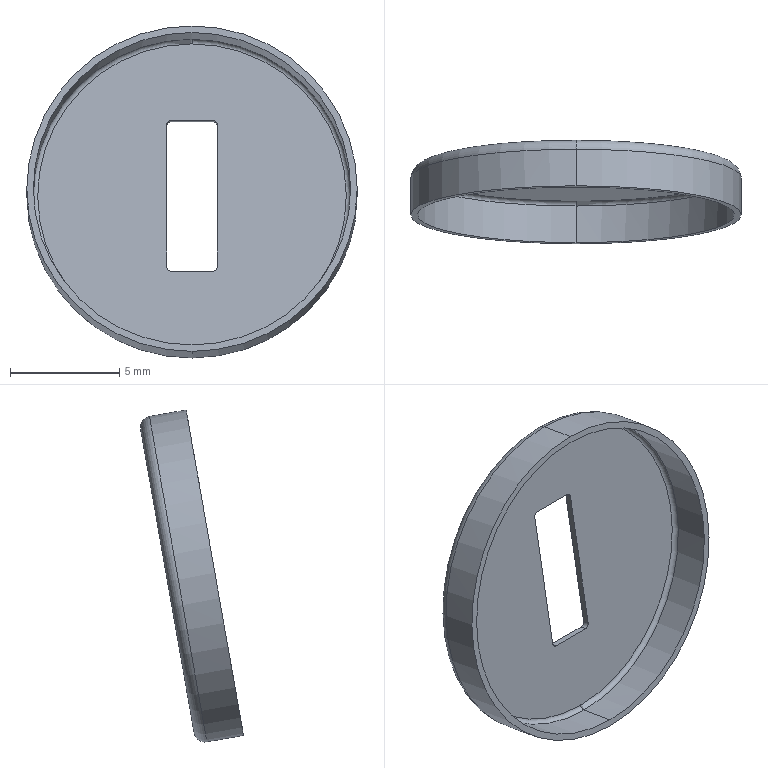Part | STEP file | _X2_751F4E45_X0_MS731-1_X2_8F_3 | 1 solid | 19 faces | box 15.1 x 4.709 x 15.173 mm | volume 73.288 mm3 | cylinder 8 | plane 7 | torus 4 | commonest cylinder face diameters 0.4 x4 14.5 x2 15.1 x2